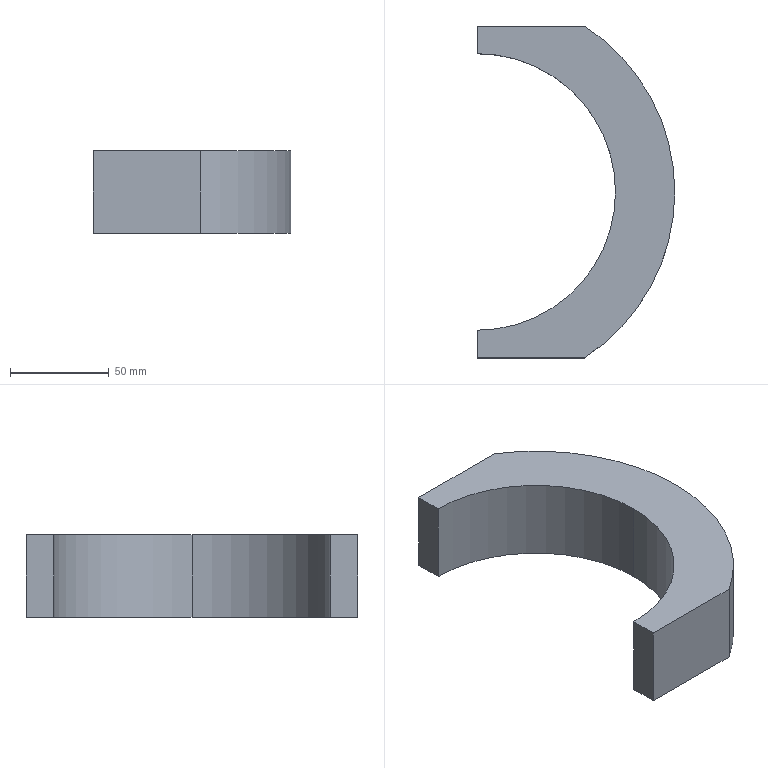Part | SolidWorks | features ICE 2, Extrusion 1 | 1 solid | 9 faces | box 100 x 168 x 42 mm | volume 287014 mm3 | plane 6 | cylinder 3 | commonest cylinder face diameters 140 x2 200 x1
STEP:
#1=CARTESIAN_POINT('',(70.,0.,0.));
#2=VERTEX_POINT('',#1);
#3=CARTESIAN_POINT('',(0.,70.,0.));
#4=VERTEX_POINT('',#3);
#5=CARTESIAN_POINT('',(0.,0.,0.));
#6=DIRECTION('',(0.,0.,1.));
#7=DIRECTION('',(1.,0.,0.));
#8=AXIS2_PLACEMENT_3D('',#5,#6,#7);
#9=CIRCLE('',#8,70.);
#10=EDGE_CURVE('',#2,#4,#9,.T.);
#11=ORIENTED_EDGE('',*,*,#10,.F.);
#12=CARTESIAN_POINT('',(70.,0.,42.));
#13=VERTEX_POINT('',#12);
#14=CARTESIAN_POINT('',(70.,0.,0.));
#15=DIRECTION('',(0.,0.,1.));
#16=VECTOR('',#15,1000.);
#17=LINE('',#14,#16);
#18=EDGE_CURVE('',#2,#13,#17,.T.);
#19=ORIENTED_EDGE('',*,*,#18,.T.);
#20=CARTESIAN_POINT('',(0.,70.,42.));
#21=VERTEX_POINT('',#20);
#22=CARTESIAN_POINT('',(0.,0.,42.));
#23=DIRECTION('',(0.,0.,1.));
#24=DIRECTION('',(1.,0.,0.));
#25=AXIS2_PLACEMENT_3D('',#22,#23,#24);
#26=CIRCLE('',#25,70.);
#27=EDGE_CURVE('',#13,#21,#26,.T.);
#28=ORIENTED_EDGE('',*,*,#27,.T.);
#29=CARTESIAN_POINT('',(0.,70.,0.));
#30=DIRECTION('',(0.,0.,1.));
#31=VECTOR('',#30,1000.);
#32=LINE('',#29,#31);
#33=EDGE_CURVE('',#4,#21,#32,.T.);
#34=ORIENTED_EDGE('',*,*,#33,.F.);
#35=EDGE_LOOP('',(#11,#19,#28,#34));
#36=FACE_OUTER_BOUND('',#35,.T.);
#37=CARTESIAN_POINT('',(0.,0.,0.));
#38=DIRECTION('',(0.,0.,1.));
#39=DIRECTION('',(1.,0.,0.));
#40=AXIS2_PLACEMENT_3D('',#37,#38,#39);
#41=CYLINDRICAL_SURFACE('',#40,70.);
#42=ADVANCED_FACE('',(#36),#41,.F.);
#43=CARTESIAN_POINT('',(54.259,-84.,0.));
#44=VERTEX_POINT('',#43);
#45=CARTESIAN_POINT('',(54.259,84.,0.));
#46=VERTEX_POINT('',#45);
#47=CARTESIAN_POINT('',(0.,0.,0.));
#48=DIRECTION('',(0.,0.,1.));
#49=DIRECTION('',(1.,0.,0.));
#50=AXIS2_PLACEMENT_3D('',#47,#48,#49);
#51=CIRCLE('',#50,100.);
#52=EDGE_CURVE('',#44,#46,#51,.T.);
#53=ORIENTED_EDGE('',*,*,#52,.T.);
#54=CARTESIAN_POINT('',(54.259,84.,42.));
#55=VERTEX_POINT('',#54);
#56=CARTESIAN_POINT('',(54.259,84.,0.));
#57=DIRECTION('',(0.,0.,1.));
#58=VECTOR('',#57,1000.);
#59=LINE('',#56,#58);
#60=EDGE_CURVE('',#46,#55,#59,.T.);
#61=ORIENTED_EDGE('',*,*,#60,.T.);
#62=CARTESIAN_POINT('',(54.259,-84.,42.));
#63=VERTEX_POINT('',#62);
#64=CARTESIAN_POINT('',(0.,0.,42.));
#65=DIRECTION('',(0.,0.,1.));
#66=DIRECTION('',(1.,0.,0.));
#67=AXIS2_PLACEMENT_3D('',#64,#65,#66);
#68=CIRCLE('',#67,100.);
#69=EDGE_CURVE('',#63,#55,#68,.T.);
#70=ORIENTED_EDGE('',*,*,#69,.F.);
#71=CARTESIAN_POINT('',(54.259,-84.,0.));
#72=DIRECTION('',(0.,0.,1.));
#73=VECTOR('',#72,1000.);
#74=LINE('',#71,#73);
#75=EDGE_CURVE('',#44,#63,#74,.T.);
#76=ORIENTED_EDGE('',*,*,#75,.F.);
#77=EDGE_LOOP('',(#53,#61,#70,#76));
#78=FACE_OUTER_BOUND('',#77,.T.);
#79=CARTESIAN_POINT('',(0.,0.,42.));
#80=DIRECTION('',(0.,0.,-1.));
#81=DIRECTION('',(-1.,0.,0.));
#82=AXIS2_PLACEMENT_3D('',#79,#80,#81);
#83=CYLINDRICAL_SURFACE('',#82,100.);
#84=ADVANCED_FACE('',(#78),#83,.T.);
#85=CARTESIAN_POINT('',(0.,-84.,42.));
#86=VERTEX_POINT('',#85);
#87=CARTESIAN_POINT('',(0.,-70.,42.));
#88=VERTEX_POINT('',#87);
#89=CARTESIAN_POINT('',(0.,-70.,42.));
#90=DIRECTION('',(0.,1.,0.));
#91=VECTOR('',#90,1000.);
#92=LINE('',#89,#91);
#93=EDGE_CURVE('',#86,#88,#92,.T.);
#94=ORIENTED_EDGE('',*,*,#93,.F.);
#95=CARTESIAN_POINT('',(-54.259,-84.,42.));
#96=DIRECTION('',(-1.,0.,0.));
#97=VECTOR('',#96,1000.);
#98=LINE('',#95,#97);
#99=EDGE_CURVE('',#63,#86,#98,.T.);
#100=ORIENTED_EDGE('',*,*,#99,.F.);
#101=ORIENTED_EDGE('',*,*,#69,.T.);
#102=CARTESIAN_POINT('',(0.,84.,42.));
#103=VERTEX_POINT('',#102);
#104=CARTESIAN_POINT('',(-54.259,84.,42.));
#105=DIRECTION('',(1.,0.,0.));
#106=VECTOR('',#105,1000.);
#107=LINE('',#104,#106);
#108=EDGE_CURVE('',#103,#55,#107,.T.);
#109=ORIENTED_EDGE('',*,*,#108,.F.);
#110=CARTESIAN_POINT('',(0.,70.,42.));
#111=DIRECTION('',(0.,1.,0.));
#112=VECTOR('',#111,1000.);
#113=LINE('',#110,#112);
#114=EDGE_CURVE('',#21,#103,#113,.T.);
#115=ORIENTED_EDGE('',*,*,#114,.F.);
#116=ORIENTED_EDGE('',*,*,#27,.F.);
#117=CARTESIAN_POINT('',(0.,0.,42.));
#118=DIRECTION('',(0.,0.,1.));
#119=DIRECTION('',(1.,0.,0.));
#120=AXIS2_PLACEMENT_3D('',#117,#118,#119);
#121=CIRCLE('',#120,70.);
#122=EDGE_CURVE('',#88,#13,#121,.T.);
#123=ORIENTED_EDGE('',*,*,#122,.F.);
#124=EDGE_LOOP('',(#94,#100,#101,#109,#115,#116,#123));
#125=FACE_OUTER_BOUND('',#124,.T.);
#126=CARTESIAN_POINT('',(0.,0.,42.));
#127=DIRECTION('',(0.,0.,1.));
#128=DIRECTION('',(1.,0.,0.));
#129=AXIS2_PLACEMENT_3D('',#126,#127,#128);
#130=PLANE('',#129);
#131=ADVANCED_FACE('',(#125),#130,.T.);
#132=CARTESIAN_POINT('',(0.,-84.,0.));
#133=VERTEX_POINT('',#132);
#134=CARTESIAN_POINT('',(-54.259,-84.,0.));
#135=DIRECTION('',(-1.,0.,0.));
#136=VECTOR('',#135,1000.);
#137=LINE('',#134,#136);
#138=EDGE_CURVE('',#44,#133,#137,.T.);
#139=ORIENTED_EDGE('',*,*,#138,.T.);
#140=CARTESIAN_POINT('',(0.,-70.,0.));
#141=VERTEX_POINT('',#140);
#142=CARTESIAN_POINT('',(0.,-70.,0.));
#143=DIRECTION('',(0.,1.,0.));
#144=VECTOR('',#143,1000.);
#145=LINE('',#142,#144);
#146=EDGE_CURVE('',#133,#141,#145,.T.);
#147=ORIENTED_EDGE('',*,*,#146,.T.);
#148=CARTESIAN_POINT('',(0.,0.,0.));
#149=DIRECTION('',(0.,0.,1.));
#150=DIRECTION('',(1.,0.,0.));
#151=AXIS2_PLACEMENT_3D('',#148,#149,#150);
#152=CIRCLE('',#151,70.);
#153=EDGE_CURVE('',#141,#2,#152,.T.);
#154=ORIENTED_EDGE('',*,*,#153,.T.);
#155=ORIENTED_EDGE('',*,*,#10,.T.);
#156=CARTESIAN_POINT('',(0.,84.,0.));
#157=VERTEX_POINT('',#156);
#158=CARTESIAN_POINT('',(0.,70.,0.));
#159=DIRECTION('',(0.,1.,0.));
#160=VECTOR('',#159,1000.);
#161=LINE('',#158,#160);
#162=EDGE_CURVE('',#4,#157,#161,.T.);
#163=ORIENTED_EDGE('',*,*,#162,.T.);
#164=CARTESIAN_POINT('',(-54.259,84.,0.));
#165=DIRECTION('',(1.,0.,0.));
#166=VECTOR('',#165,1000.);
#167=LINE('',#164,#166);
#168=EDGE_CURVE('',#157,#46,#167,.T.);
#169=ORIENTED_EDGE('',*,*,#168,.T.);
#170=ORIENTED_EDGE('',*,*,#52,.F.);
#171=EDGE_LOOP('',(#139,#147,#154,#155,#163,#169,#170));
#172=FACE_OUTER_BOUND('',#171,.T.);
#173=CARTESIAN_POINT('',(0.,0.,0.));
#174=DIRECTION('',(0.,0.,1.));
#175=DIRECTION('',(1.,0.,0.));
#176=AXIS2_PLACEMENT_3D('',#173,#174,#175);
#177=PLANE('',#176);
#178=ADVANCED_FACE('',(#172),#177,.F.);
#179=ORIENTED_EDGE('',*,*,#99,.T.);
#180=CARTESIAN_POINT('',(0.,-84.,0.));
#181=DIRECTION('',(0.,0.,1.));
#182=VECTOR('',#181,1000.);
#183=LINE('',#180,#182);
#184=EDGE_CURVE('',#133,#86,#183,.T.);
#185=ORIENTED_EDGE('',*,*,#184,.F.);
#186=ORIENTED_EDGE('',*,*,#138,.F.);
#187=ORIENTED_EDGE('',*,*,#75,.T.);
#188=EDGE_LOOP('',(#179,#185,#186,#187));
#189=FACE_OUTER_BOUND('',#188,.T.);
#190=CARTESIAN_POINT('',(-54.259,-84.,0.));
#191=DIRECTION('',(0.,1.,0.));
#192=DIRECTION('',(-1.,0.,0.));
#193=AXIS2_PLACEMENT_3D('',#190,#191,#192);
#194=PLANE('',#193);
#195=ADVANCED_FACE('',(#189),#194,.F.);
#196=ORIENTED_EDGE('',*,*,#168,.F.);
#197=CARTESIAN_POINT('',(0.,84.,0.));
#198=DIRECTION('',(0.,0.,1.));
#199=VECTOR('',#198,1000.);
#200=LINE('',#197,#199);
#201=EDGE_CURVE('',#157,#103,#200,.T.);
#202=ORIENTED_EDGE('',*,*,#201,.T.);
#203=ORIENTED_EDGE('',*,*,#108,.T.);
#204=ORIENTED_EDGE('',*,*,#60,.F.);
#205=EDGE_LOOP('',(#196,#202,#203,#204));
#206=FACE_OUTER_BOUND('',#205,.T.);
#207=CARTESIAN_POINT('',(-54.259,84.,0.));
#208=DIRECTION('',(0.,-1.,0.));
#209=DIRECTION('',(1.,0.,0.));
#210=AXIS2_PLACEMENT_3D('',#207,#208,#209);
#211=PLANE('',#210);
#212=ADVANCED_FACE('',(#206),#211,.F.);
#213=ORIENTED_EDGE('',*,*,#18,.F.);
#214=ORIENTED_EDGE('',*,*,#153,.F.);
#215=CARTESIAN_POINT('',(0.,-70.,0.));
#216=DIRECTION('',(0.,0.,1.));
#217=VECTOR('',#216,1000.);
#218=LINE('',#215,#217);
#219=EDGE_CURVE('',#141,#88,#218,.T.);
#220=ORIENTED_EDGE('',*,*,#219,.T.);
#221=ORIENTED_EDGE('',*,*,#122,.T.);
#222=EDGE_LOOP('',(#213,#214,#220,#221));
#223=FACE_OUTER_BOUND('',#222,.T.);
#224=CARTESIAN_POINT('',(0.,0.,0.));
#225=DIRECTION('',(0.,0.,1.));
#226=DIRECTION('',(1.,0.,0.));
#227=AXIS2_PLACEMENT_3D('',#224,#225,#226);
#228=CYLINDRICAL_SURFACE('',#227,70.);
#229=ADVANCED_FACE('',(#223),#228,.F.);
#230=ORIENTED_EDGE('',*,*,#93,.T.);
#231=ORIENTED_EDGE('',*,*,#219,.F.);
#232=ORIENTED_EDGE('',*,*,#146,.F.);
#233=ORIENTED_EDGE('',*,*,#184,.T.);
#234=EDGE_LOOP('',(#230,#231,#232,#233));
#235=FACE_OUTER_BOUND('',#234,.T.);
#236=CARTESIAN_POINT('',(0.,-70.,0.));
#237=DIRECTION('',(1.,0.,0.));
#238=DIRECTION('',(0.,0.,-1.));
#239=AXIS2_PLACEMENT_3D('',#236,#237,#238);
#240=PLANE('',#239);
#241=ADVANCED_FACE('',(#235),#240,.F.);
#242=ORIENTED_EDGE('',*,*,#114,.T.);
#243=ORIENTED_EDGE('',*,*,#201,.F.);
#244=ORIENTED_EDGE('',*,*,#162,.F.);
#245=ORIENTED_EDGE('',*,*,#33,.T.);
#246=EDGE_LOOP('',(#242,#243,#244,#245));
#247=FACE_OUTER_BOUND('',#246,.T.);
#248=CARTESIAN_POINT('',(0.,70.,0.));
#249=DIRECTION('',(1.,0.,0.));
#250=DIRECTION('',(0.,0.,-1.));
#251=AXIS2_PLACEMENT_3D('',#248,#249,#250);
#252=PLANE('',#251);
#253=ADVANCED_FACE('',(#247),#252,.F.);
#254=CLOSED_SHELL('',(#42,#84,#131,#178,#195,#212,#229,#241,#253));
#255=MANIFOLD_SOLID_BREP('',#254);
#256=CARTESIAN_POINT('',(0.,0.,0.));
#257=DIRECTION('',(0.,0.,1.));
#258=DIRECTION('',(1.,0.,0.));
#259=AXIS2_PLACEMENT_3D('',#256,#257,#258);
#260=(LENGTH_UNIT()NAMED_UNIT(*)SI_UNIT(.MILLI.,.METRE.));
#261=UNCERTAINTY_MEASURE_WITH_UNIT(LENGTH_MEASURE(0.00001),#260,'','');
#262=(NAMED_UNIT(*)PLANE_ANGLE_UNIT()SI_UNIT($,.RADIAN.));
#263=(NAMED_UNIT(*)SI_UNIT($,.STERADIAN.)SOLID_ANGLE_UNIT());
#264=(GEOMETRIC_REPRESENTATION_CONTEXT(3)GLOBAL_UNCERTAINTY_ASSIGNED_CONTEXT((#261))GLOBAL_UNIT_ASSIGNED_CONTEXT((#260,#262,#263))REPRESENTATION_CONTEXT('',''));
#265=ADVANCED_BREP_SHAPE_REPRESENTATION('',(#255,#259),#264);